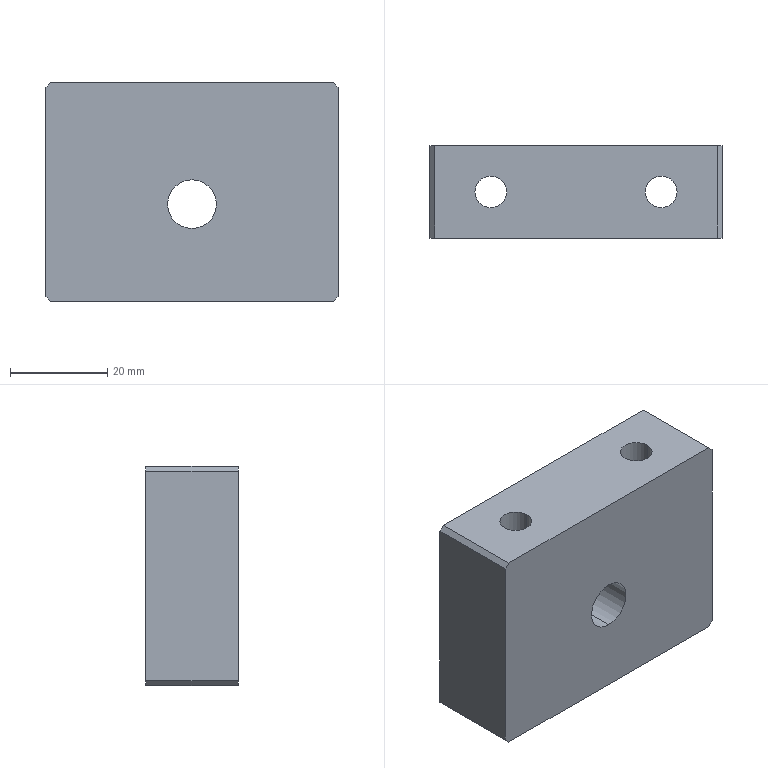Part | STEP file | 1 solid | 29 faces | box 60 x 19 x 45 mm | volume 39956 mm3 | cylinder 14 | plane 13 | cone 2 | commonest cylinder face diameters 6.5 x4 12 x4 4.2 x2 10 x2 20 x2